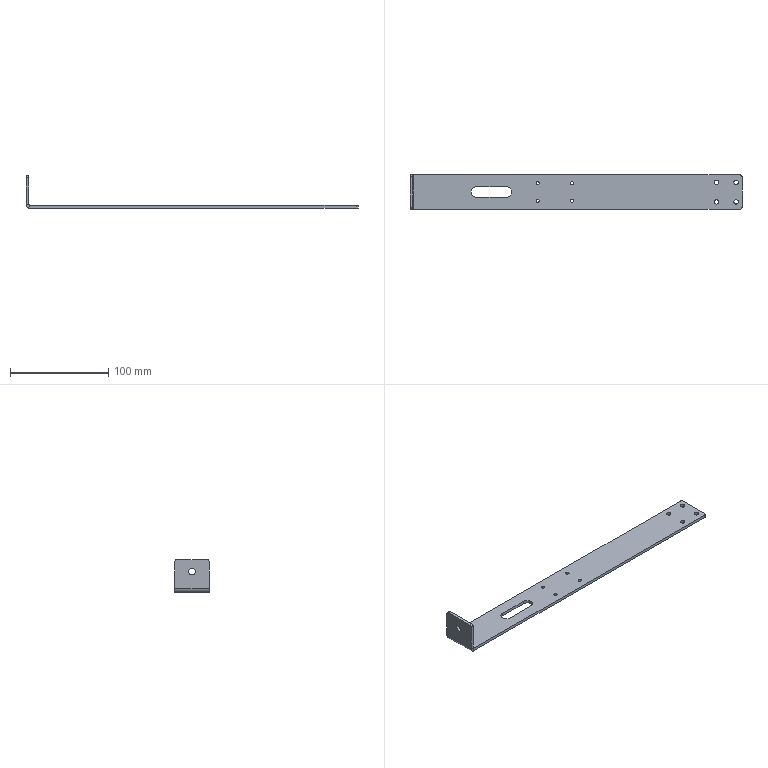Part | NX | features BREP 1 | 1 solid | 41 faces | box 338 x 35 x 33 mm | volume 36858 mm3 | cylinder 27 | plane 14 | commonest cylinder face diameters 3.3 x8 4.5 x8 4 x4 11 x3 6.6 x2 1.473 x1
STEP:
#1=CARTESIAN_POINT('',(-169.,0.,14.7));
#2=VERTEX_POINT('',#1);
#3=CARTESIAN_POINT('',(-166.,0.,14.7));
#4=VERTEX_POINT('',#3);
#5=CARTESIAN_POINT('',(-169.,0.,14.7));
#6=DIRECTION('',(-1.,0.,0.));
#7=VECTOR('',#6,1000.);
#8=LINE('',#5,#7);
#9=EDGE_CURVE('',#2,#4,#8,.F.);
#10=ORIENTED_EDGE('',*,*,#9,.T.);
#11=CARTESIAN_POINT('',(-166.,0.,21.3));
#12=VERTEX_POINT('',#11);
#13=CARTESIAN_POINT('',(-166.,0.,18.));
#14=DIRECTION('',(1.,0.,0.));
#15=DIRECTION('',(0.,0.,-1.));
#16=AXIS2_PLACEMENT_3D('',#13,#14,#15);
#17=CIRCLE('',#16,3.3);
#18=EDGE_CURVE('',#4,#12,#17,.T.);
#19=ORIENTED_EDGE('',*,*,#18,.T.);
#20=CARTESIAN_POINT('',(-169.,0.,21.3));
#21=VERTEX_POINT('',#20);
#22=CARTESIAN_POINT('',(-169.,0.,21.3));
#23=DIRECTION('',(-1.,0.,0.));
#24=VECTOR('',#23,1000.);
#25=LINE('',#22,#24);
#26=EDGE_CURVE('',#21,#12,#25,.F.);
#27=ORIENTED_EDGE('',*,*,#26,.F.);
#28=CARTESIAN_POINT('',(-169.,0.,18.));
#29=DIRECTION('',(-1.,0.,0.));
#30=DIRECTION('',(0.,0.,1.));
#31=AXIS2_PLACEMENT_3D('',#28,#29,#30);
#32=CIRCLE('',#31,3.3);
#33=EDGE_CURVE('',#21,#2,#32,.T.);
#34=ORIENTED_EDGE('',*,*,#33,.T.);
#35=EDGE_LOOP('',(#10,#19,#27,#34));
#36=FACE_BOUND('',#35,.T.);
#37=CARTESIAN_POINT('',(-169.,0.,18.));
#38=DIRECTION('',(-1.,0.,0.));
#39=DIRECTION('',(0.,0.,1.));
#40=AXIS2_PLACEMENT_3D('',#37,#38,#39);
#41=CYLINDRICAL_SURFACE('',#40,3.3);
#42=ADVANCED_FACE('',(#36),#41,.F.);
#43=CARTESIAN_POINT('',(167.,17.5,-3.));
#44=VERTEX_POINT('',#43);
#45=CARTESIAN_POINT('',(169.,15.5,-3.));
#46=VERTEX_POINT('',#45);
#47=CARTESIAN_POINT('',(167.,15.5,-3.));
#48=DIRECTION('',(0.,0.,-1.));
#49=DIRECTION('',(1.,0.,0.));
#50=AXIS2_PLACEMENT_3D('',#47,#48,#49);
#51=CIRCLE('',#50,2.);
#52=EDGE_CURVE('',#44,#46,#51,.T.);
#53=ORIENTED_EDGE('',*,*,#52,.F.);
#54=CARTESIAN_POINT('',(167.,17.5,0.));
#55=VERTEX_POINT('',#54);
#56=CARTESIAN_POINT('',(167.,17.5,-3.));
#57=DIRECTION('',(0.,0.,-1.));
#58=VECTOR('',#57,1000.);
#59=LINE('',#56,#58);
#60=EDGE_CURVE('',#55,#44,#59,.T.);
#61=ORIENTED_EDGE('',*,*,#60,.F.);
#62=CARTESIAN_POINT('',(169.,15.5,0.));
#63=VERTEX_POINT('',#62);
#64=CARTESIAN_POINT('',(167.,15.5,0.));
#65=DIRECTION('',(0.,0.,1.));
#66=DIRECTION('',(1.,0.,0.));
#67=AXIS2_PLACEMENT_3D('',#64,#65,#66);
#68=CIRCLE('',#67,2.);
#69=EDGE_CURVE('',#63,#55,#68,.T.);
#70=ORIENTED_EDGE('',*,*,#69,.F.);
#71=CARTESIAN_POINT('',(169.,15.5,-3.));
#72=DIRECTION('',(0.,0.,1.));
#73=VECTOR('',#72,1000.);
#74=LINE('',#71,#73);
#75=EDGE_CURVE('',#46,#63,#74,.T.);
#76=ORIENTED_EDGE('',*,*,#75,.F.);
#77=EDGE_LOOP('',(#53,#61,#70,#76));
#78=FACE_BOUND('',#77,.T.);
#79=CARTESIAN_POINT('',(167.,15.5,-3.));
#80=DIRECTION('',(0.,0.,1.));
#81=DIRECTION('',(1.,0.,0.));
#82=AXIS2_PLACEMENT_3D('',#79,#80,#81);
#83=CYLINDRICAL_SURFACE('',#82,2.);
#84=ADVANCED_FACE('',(#78),#83,.T.);
#85=CARTESIAN_POINT('',(169.,-15.5,-3.));
#86=VERTEX_POINT('',#85);
#87=CARTESIAN_POINT('',(167.,-17.5,-3.));
#88=VERTEX_POINT('',#87);
#89=CARTESIAN_POINT('',(167.,-15.5,-3.));
#90=DIRECTION('',(0.,0.,-1.));
#91=DIRECTION('',(1.,0.,0.));
#92=AXIS2_PLACEMENT_3D('',#89,#90,#91);
#93=CIRCLE('',#92,2.);
#94=EDGE_CURVE('',#86,#88,#93,.T.);
#95=ORIENTED_EDGE('',*,*,#94,.F.);
#96=CARTESIAN_POINT('',(169.,-15.5,0.));
#97=VERTEX_POINT('',#96);
#98=CARTESIAN_POINT('',(169.,-15.5,-3.));
#99=DIRECTION('',(0.,0.,-1.));
#100=VECTOR('',#99,1000.);
#101=LINE('',#98,#100);
#102=EDGE_CURVE('',#97,#86,#101,.T.);
#103=ORIENTED_EDGE('',*,*,#102,.F.);
#104=CARTESIAN_POINT('',(167.,-17.5,0.));
#105=VERTEX_POINT('',#104);
#106=CARTESIAN_POINT('',(167.,-15.5,0.));
#107=DIRECTION('',(0.,0.,1.));
#108=DIRECTION('',(1.,0.,0.));
#109=AXIS2_PLACEMENT_3D('',#106,#107,#108);
#110=CIRCLE('',#109,2.);
#111=EDGE_CURVE('',#105,#97,#110,.T.);
#112=ORIENTED_EDGE('',*,*,#111,.F.);
#113=CARTESIAN_POINT('',(167.,-17.5,-3.));
#114=DIRECTION('',(0.,0.,1.));
#115=VECTOR('',#114,1000.);
#116=LINE('',#113,#115);
#117=EDGE_CURVE('',#88,#105,#116,.T.);
#118=ORIENTED_EDGE('',*,*,#117,.F.);
#119=EDGE_LOOP('',(#95,#103,#112,#118));
#120=FACE_BOUND('',#119,.T.);
#121=CARTESIAN_POINT('',(167.,-15.5,-3.));
#122=DIRECTION('',(0.,0.,1.));
#123=DIRECTION('',(1.,0.,0.));
#124=AXIS2_PLACEMENT_3D('',#121,#122,#123);
#125=CYLINDRICAL_SURFACE('',#124,2.);
#126=ADVANCED_FACE('',(#120),#125,.T.);
#127=CARTESIAN_POINT('',(-169.,15.5,30.));
#128=VERTEX_POINT('',#127);
#129=CARTESIAN_POINT('',(-169.,17.5,28.));
#130=VERTEX_POINT('',#129);
#131=CARTESIAN_POINT('',(-169.,15.5,28.));
#132=DIRECTION('',(-1.,0.,0.));
#133=DIRECTION('',(0.,0.,-1.));
#134=AXIS2_PLACEMENT_3D('',#131,#132,#133);
#135=CIRCLE('',#134,2.);
#136=EDGE_CURVE('',#128,#130,#135,.T.);
#137=ORIENTED_EDGE('',*,*,#136,.F.);
#138=CARTESIAN_POINT('',(-166.,15.5,30.));
#139=VERTEX_POINT('',#138);
#140=CARTESIAN_POINT('',(-169.,15.5,30.));
#141=DIRECTION('',(-1.,0.,0.));
#142=VECTOR('',#141,1000.);
#143=LINE('',#140,#142);
#144=EDGE_CURVE('',#139,#128,#143,.T.);
#145=ORIENTED_EDGE('',*,*,#144,.F.);
#146=CARTESIAN_POINT('',(-166.,17.5,28.));
#147=VERTEX_POINT('',#146);
#148=CARTESIAN_POINT('',(-166.,15.5,28.));
#149=DIRECTION('',(1.,0.,0.));
#150=DIRECTION('',(0.,0.,-1.));
#151=AXIS2_PLACEMENT_3D('',#148,#149,#150);
#152=CIRCLE('',#151,2.);
#153=EDGE_CURVE('',#147,#139,#152,.T.);
#154=ORIENTED_EDGE('',*,*,#153,.F.);
#155=CARTESIAN_POINT('',(-169.,17.5,28.));
#156=DIRECTION('',(1.,0.,0.));
#157=VECTOR('',#156,1000.);
#158=LINE('',#155,#157);
#159=EDGE_CURVE('',#130,#147,#158,.T.);
#160=ORIENTED_EDGE('',*,*,#159,.F.);
#161=EDGE_LOOP('',(#137,#145,#154,#160));
#162=FACE_BOUND('',#161,.T.);
#163=CARTESIAN_POINT('',(-169.,15.5,28.));
#164=DIRECTION('',(1.,0.,0.));
#165=DIRECTION('',(0.,0.,-1.));
#166=AXIS2_PLACEMENT_3D('',#163,#164,#165);
#167=CYLINDRICAL_SURFACE('',#166,2.);
#168=ADVANCED_FACE('',(#162),#167,.T.);
#169=CARTESIAN_POINT('',(-169.,-17.5,28.));
#170=VERTEX_POINT('',#169);
#171=CARTESIAN_POINT('',(-169.,-15.5,30.));
#172=VERTEX_POINT('',#171);
#173=CARTESIAN_POINT('',(-169.,-15.5,28.));
#174=DIRECTION('',(-1.,0.,0.));
#175=DIRECTION('',(0.,0.,-1.));
#176=AXIS2_PLACEMENT_3D('',#173,#174,#175);
#177=CIRCLE('',#176,2.);
#178=EDGE_CURVE('',#170,#172,#177,.T.);
#179=ORIENTED_EDGE('',*,*,#178,.F.);
#180=CARTESIAN_POINT('',(-166.,-17.5,28.));
#181=VERTEX_POINT('',#180);
#182=CARTESIAN_POINT('',(-169.,-17.5,28.));
#183=DIRECTION('',(-1.,0.,0.));
#184=VECTOR('',#183,1000.);
#185=LINE('',#182,#184);
#186=EDGE_CURVE('',#181,#170,#185,.T.);
#187=ORIENTED_EDGE('',*,*,#186,.F.);
#188=CARTESIAN_POINT('',(-166.,-15.5,30.));
#189=VERTEX_POINT('',#188);
#190=CARTESIAN_POINT('',(-166.,-15.5,28.));
#191=DIRECTION('',(1.,0.,0.));
#192=DIRECTION('',(0.,0.,-1.));
#193=AXIS2_PLACEMENT_3D('',#190,#191,#192);
#194=CIRCLE('',#193,2.);
#195=EDGE_CURVE('',#189,#181,#194,.T.);
#196=ORIENTED_EDGE('',*,*,#195,.F.);
#197=CARTESIAN_POINT('',(-169.,-15.5,30.));
#198=DIRECTION('',(1.,0.,0.));
#199=VECTOR('',#198,1000.);
#200=LINE('',#197,#199);
#201=EDGE_CURVE('',#172,#189,#200,.T.);
#202=ORIENTED_EDGE('',*,*,#201,.F.);
#203=EDGE_LOOP('',(#179,#187,#196,#202));
#204=FACE_BOUND('',#203,.T.);
#205=CARTESIAN_POINT('',(-169.,-15.5,28.));
#206=DIRECTION('',(1.,0.,0.));
#207=DIRECTION('',(0.,0.,-1.));
#208=AXIS2_PLACEMENT_3D('',#205,#206,#207);
#209=CYLINDRICAL_SURFACE('',#208,2.);
#210=ADVANCED_FACE('',(#204),#209,.T.);
#211=CARTESIAN_POINT('',(-71.,5.5,0.));
#212=VERTEX_POINT('',#211);
#213=CARTESIAN_POINT('',(-101.,5.5,0.));
#214=VERTEX_POINT('',#213);
#215=CARTESIAN_POINT('',(0.,5.5,0.));
#216=DIRECTION('',(-1.,0.,0.));
#217=VECTOR('',#216,1000.);
#218=LINE('',#215,#217);
#219=EDGE_CURVE('',#212,#214,#218,.T.);
#220=ORIENTED_EDGE('',*,*,#219,.T.);
#221=CARTESIAN_POINT('',(-101.,5.5,-3.));
#222=VERTEX_POINT('',#221);
#223=CARTESIAN_POINT('',(-101.,5.5,-3.));
#224=DIRECTION('',(0.,0.,-1.));
#225=VECTOR('',#224,1000.);
#226=LINE('',#223,#225);
#227=EDGE_CURVE('',#214,#222,#226,.T.);
#228=ORIENTED_EDGE('',*,*,#227,.T.);
#229=CARTESIAN_POINT('',(-71.,5.5,-3.));
#230=VERTEX_POINT('',#229);
#231=CARTESIAN_POINT('',(-101.,5.5,-3.));
#232=DIRECTION('',(1.,0.,0.));
#233=VECTOR('',#232,1000.);
#234=LINE('',#231,#233);
#235=EDGE_CURVE('',#222,#230,#234,.T.);
#236=ORIENTED_EDGE('',*,*,#235,.T.);
#237=CARTESIAN_POINT('',(-71.,5.5,-3.));
#238=DIRECTION('',(0.,0.,1.));
#239=VECTOR('',#238,1000.);
#240=LINE('',#237,#239);
#241=EDGE_CURVE('',#230,#212,#240,.T.);
#242=ORIENTED_EDGE('',*,*,#241,.T.);
#243=EDGE_LOOP('',(#220,#228,#236,#242));
#244=FACE_BOUND('',#243,.T.);
#245=CARTESIAN_POINT('',(-101.,5.5,-3.));
#246=DIRECTION('',(0.,1.,0.));
#247=DIRECTION('',(0.,0.,1.));
#248=AXIS2_PLACEMENT_3D('',#245,#246,#247);
#249=PLANE('',#248);
#250=ADVANCED_FACE('',(#244),#249,.F.);
#251=CARTESIAN_POINT('',(-101.,-5.5,0.));
#252=VERTEX_POINT('',#251);
#253=CARTESIAN_POINT('',(-71.,-5.5,0.));
#254=VERTEX_POINT('',#253);
#255=CARTESIAN_POINT('',(0.,-5.5,0.));
#256=DIRECTION('',(1.,0.,0.));
#257=VECTOR('',#256,1000.);
#258=LINE('',#255,#257);
#259=EDGE_CURVE('',#252,#254,#258,.T.);
#260=ORIENTED_EDGE('',*,*,#259,.T.);
#261=CARTESIAN_POINT('',(-71.,-5.5,-3.));
#262=VERTEX_POINT('',#261);
#263=CARTESIAN_POINT('',(-71.,-5.5,-3.));
#264=DIRECTION('',(0.,0.,-1.));
#265=VECTOR('',#264,1000.);
#266=LINE('',#263,#265);
#267=EDGE_CURVE('',#254,#262,#266,.T.);
#268=ORIENTED_EDGE('',*,*,#267,.T.);
#269=CARTESIAN_POINT('',(-101.,-5.5,-3.));
#270=VERTEX_POINT('',#269);
#271=CARTESIAN_POINT('',(-101.,-5.5,-3.));
#272=DIRECTION('',(1.,0.,0.));
#273=VECTOR('',#272,1000.);
#274=LINE('',#271,#273);
#275=EDGE_CURVE('',#270,#262,#274,.T.);
#276=ORIENTED_EDGE('',*,*,#275,.F.);
#277=CARTESIAN_POINT('',(-101.,-5.5,-3.));
#278=DIRECTION('',(0.,0.,1.));
#279=VECTOR('',#278,1000.);
#280=LINE('',#277,#279);
#281=EDGE_CURVE('',#270,#252,#280,.T.);
#282=ORIENTED_EDGE('',*,*,#281,.T.);
#283=EDGE_LOOP('',(#260,#268,#276,#282));
#284=FACE_BOUND('',#283,.T.);
#285=CARTESIAN_POINT('',(-101.,-5.5,-3.));
#286=DIRECTION('',(0.,-1.,0.));
#287=DIRECTION('',(0.,0.,-1.));
#288=AXIS2_PLACEMENT_3D('',#285,#286,#287);
#289=PLANE('',#288);
#290=ADVANCED_FACE('',(#284),#289,.F.);
#291=CARTESIAN_POINT('',(-106.5,0.,0.));
#292=VERTEX_POINT('',#291);
#293=CARTESIAN_POINT('',(-106.5,0.,-3.));
#294=VERTEX_POINT('',#293);
#295=CARTESIAN_POINT('',(-106.5,0.,-3.));
#296=DIRECTION('',(0.,0.,-1.));
#297=VECTOR('',#296,1000.);
#298=LINE('',#295,#297);
#299=EDGE_CURVE('',#292,#294,#298,.T.);
#300=ORIENTED_EDGE('',*,*,#299,.F.);
#301=CARTESIAN_POINT('',(-101.,0.,0.));
#302=DIRECTION('',(0.,0.,1.));
#303=DIRECTION('',(1.,0.,0.));
#304=AXIS2_PLACEMENT_3D('',#301,#302,#303);
#305=CIRCLE('',#304,5.5);
#306=EDGE_CURVE('',#292,#252,#305,.T.);
#307=ORIENTED_EDGE('',*,*,#306,.T.);
#308=ORIENTED_EDGE('',*,*,#281,.F.);
#309=CARTESIAN_POINT('',(-101.,0.,-3.));
#310=DIRECTION('',(0.,0.,-1.));
#311=DIRECTION('',(-1.,0.,0.));
#312=AXIS2_PLACEMENT_3D('',#309,#310,#311);
#313=CIRCLE('',#312,5.5);
#314=EDGE_CURVE('',#270,#294,#313,.T.);
#315=ORIENTED_EDGE('',*,*,#314,.T.);
#316=EDGE_LOOP('',(#300,#307,#308,#315));
#317=FACE_BOUND('',#316,.T.);
#318=CARTESIAN_POINT('',(-101.,0.,-3.));
#319=DIRECTION('',(0.,0.,-1.));
#320=DIRECTION('',(-1.,0.,0.));
#321=AXIS2_PLACEMENT_3D('',#318,#319,#320);
#322=CYLINDRICAL_SURFACE('',#321,5.5);
#323=ADVANCED_FACE('',(#317),#322,.F.);
#324=CARTESIAN_POINT('',(-71.,0.,0.));
#325=DIRECTION('',(0.,0.,1.));
#326=DIRECTION('',(1.,0.,0.));
#327=AXIS2_PLACEMENT_3D('',#324,#325,#326);
#328=CIRCLE('',#327,5.5);
#329=EDGE_CURVE('',#254,#212,#328,.T.);
#330=ORIENTED_EDGE('',*,*,#329,.T.);
#331=ORIENTED_EDGE('',*,*,#241,.F.);
#332=CARTESIAN_POINT('',(-71.,0.,-3.));
#333=DIRECTION('',(0.,0.,-1.));
#334=DIRECTION('',(-1.,0.,0.));
#335=AXIS2_PLACEMENT_3D('',#332,#333,#334);
#336=CIRCLE('',#335,5.5);
#337=EDGE_CURVE('',#230,#262,#336,.T.);
#338=ORIENTED_EDGE('',*,*,#337,.T.);
#339=ORIENTED_EDGE('',*,*,#267,.F.);
#340=EDGE_LOOP('',(#330,#331,#338,#339));
#341=FACE_BOUND('',#340,.T.);
#342=CARTESIAN_POINT('',(-71.,0.,-3.));
#343=DIRECTION('',(0.,0.,-1.));
#344=DIRECTION('',(-1.,0.,0.));
#345=AXIS2_PLACEMENT_3D('',#342,#343,#344);
#346=CYLINDRICAL_SURFACE('',#345,5.5);
#347=ADVANCED_FACE('',(#341),#346,.F.);
#348=CARTESIAN_POINT('',(-40.65,9.,0.));
#349=VERTEX_POINT('',#348);
#350=CARTESIAN_POINT('',(-40.65,9.,-3.));
#351=VERTEX_POINT('',#350);
#352=CARTESIAN_POINT('',(-40.65,9.,0.));
#353=DIRECTION('',(0.,0.,1.));
#354=VECTOR('',#353,1000.);
#355=LINE('',#352,#354);
#356=EDGE_CURVE('',#349,#351,#355,.F.);
#357=ORIENTED_EDGE('',*,*,#356,.T.);
#358=CARTESIAN_POINT('',(-37.35,9.,-3.));
#359=VERTEX_POINT('',#358);
#360=CARTESIAN_POINT('',(-39.,9.,-3.));
#361=DIRECTION('',(0.,0.,1.));
#362=DIRECTION('',(1.,0.,0.));
#363=AXIS2_PLACEMENT_3D('',#360,#361,#362);
#364=CIRCLE('',#363,1.65);
#365=EDGE_CURVE('',#359,#351,#364,.T.);
#366=ORIENTED_EDGE('',*,*,#365,.F.);
#367=CARTESIAN_POINT('',(-37.35,9.,0.));
#368=VERTEX_POINT('',#367);
#369=CARTESIAN_POINT('',(-37.35,9.,0.));
#370=DIRECTION('',(0.,0.,1.));
#371=VECTOR('',#370,1000.);
#372=LINE('',#369,#371);
#373=EDGE_CURVE('',#368,#359,#372,.F.);
#374=ORIENTED_EDGE('',*,*,#373,.F.);
#375=CARTESIAN_POINT('',(-39.,9.,0.));
#376=DIRECTION('',(0.,0.,1.));
#377=DIRECTION('',(1.,0.,0.));
#378=AXIS2_PLACEMENT_3D('',#375,#376,#377);
#379=CIRCLE('',#378,1.65);
#380=EDGE_CURVE('',#368,#349,#379,.T.);
#381=ORIENTED_EDGE('',*,*,#380,.T.);
#382=EDGE_LOOP('',(#357,#366,#374,#381));
#383=FACE_BOUND('',#382,.T.);
#384=CARTESIAN_POINT('',(-39.,9.,0.));
#385=DIRECTION('',(0.,0.,1.));
#386=DIRECTION('',(1.,0.,0.));
#387=AXIS2_PLACEMENT_3D('',#384,#385,#386);
#388=CYLINDRICAL_SURFACE('',#387,1.65);
#389=ADVANCED_FACE('',(#383),#388,.F.);
#390=CARTESIAN_POINT('',(-40.65,-9.,0.));
#391=VERTEX_POINT('',#390);
#392=CARTESIAN_POINT('',(-40.65,-9.,-3.));
#393=VERTEX_POINT('',#392);
#394=CARTESIAN_POINT('',(-40.65,-9.,0.));
#395=DIRECTION('',(0.,0.,1.));
#396=VECTOR('',#395,1000.);
#397=LINE('',#394,#396);
#398=EDGE_CURVE('',#391,#393,#397,.F.);
#399=ORIENTED_EDGE('',*,*,#398,.T.);
#400=CARTESIAN_POINT('',(-37.35,-9.,-3.));
#401=VERTEX_POINT('',#400);
#402=CARTESIAN_POINT('',(-39.,-9.,-3.));
#403=DIRECTION('',(0.,0.,1.));
#404=DIRECTION('',(1.,0.,0.));
#405=AXIS2_PLACEMENT_3D('',#402,#403,#404);
#406=CIRCLE('',#405,1.65);
#407=EDGE_CURVE('',#401,#393,#406,.T.);
#408=ORIENTED_EDGE('',*,*,#407,.F.);
#409=CARTESIAN_POINT('',(-37.35,-9.,0.));
#410=VERTEX_POINT('',#409);
#411=CARTESIAN_POINT('',(-37.35,-9.,0.));
#412=DIRECTION('',(0.,0.,1.));
#413=VECTOR('',#412,1000.);
#414=LINE('',#411,#413);
#415=EDGE_CURVE('',#410,#401,#414,.F.);
#416=ORIENTED_EDGE('',*,*,#415,.F.);
#417=CARTESIAN_POINT('',(-39.,-9.,0.));
#418=DIRECTION('',(0.,0.,1.));
#419=DIRECTION('',(1.,0.,0.));
#420=AXIS2_PLACEMENT_3D('',#417,#418,#419);
#421=CIRCLE('',#420,1.65);
#422=EDGE_CURVE('',#410,#391,#421,.T.);
#423=ORIENTED_EDGE('',*,*,#422,.T.);
#424=EDGE_LOOP('',(#399,#408,#416,#423));
#425=FACE_BOUND('',#424,.T.);
#426=CARTESIAN_POINT('',(-39.,-9.,0.));
#427=DIRECTION('',(0.,0.,1.));
#428=DIRECTION('',(1.,0.,0.));
#429=AXIS2_PLACEMENT_3D('',#426,#427,#428);
#430=CYLINDRICAL_SURFACE('',#429,1.65);
#431=ADVANCED_FACE('',(#425),#430,.F.);
#432=CARTESIAN_POINT('',(-5.65,-9.,0.));
#433=VERTEX_POINT('',#432);
#434=CARTESIAN_POINT('',(-5.65,-9.,-3.));
#435=VERTEX_POINT('',#434);
#436=CARTESIAN_POINT('',(-5.65,-9.,0.));
#437=DIRECTION('',(0.,0.,1.));
#438=VECTOR('',#437,1000.);
#439=LINE('',#436,#438);
#440=EDGE_CURVE('',#433,#435,#439,.F.);
#441=ORIENTED_EDGE('',*,*,#440,.T.);
#442=CARTESIAN_POINT('',(-2.35,-9.,-3.));
#443=VERTEX_POINT('',#442);
#444=CARTESIAN_POINT('',(-4.,-9.,-3.));
#445=DIRECTION('',(0.,0.,1.));
#446=DIRECTION('',(1.,0.,0.));
#447=AXIS2_PLACEMENT_3D('',#444,#445,#446);
#448=CIRCLE('',#447,1.65);
#449=EDGE_CURVE('',#443,#435,#448,.T.);
#450=ORIENTED_EDGE('',*,*,#449,.F.);
#451=CARTESIAN_POINT('',(-2.35,-9.,0.));
#452=VERTEX_POINT('',#451);
#453=CARTESIAN_POINT('',(-2.35,-9.,0.));
#454=DIRECTION('',(0.,0.,1.));
#455=VECTOR('',#454,1000.);
#456=LINE('',#453,#455);
#457=EDGE_CURVE('',#452,#443,#456,.F.);
#458=ORIENTED_EDGE('',*,*,#457,.F.);
#459=CARTESIAN_POINT('',(-4.,-9.,0.));
#460=DIRECTION('',(0.,0.,1.));
#461=DIRECTION('',(1.,0.,0.));
#462=AXIS2_PLACEMENT_3D('',#459,#460,#461);
#463=CIRCLE('',#462,1.65);
#464=EDGE_CURVE('',#452,#433,#463,.T.);
#465=ORIENTED_EDGE('',*,*,#464,.T.);
#466=EDGE_LOOP('',(#441,#450,#458,#465));
#467=FACE_BOUND('',#466,.T.);
#468=CARTESIAN_POINT('',(-4.,-9.,0.));
#469=DIRECTION('',(0.,0.,1.));
#470=DIRECTION('',(1.,0.,0.));
#471=AXIS2_PLACEMENT_3D('',#468,#469,#470);
#472=CYLINDRICAL_SURFACE('',#471,1.65);
#473=ADVANCED_FACE('',(#467),#472,.F.);
#474=CARTESIAN_POINT('',(-5.65,9.,0.));
#475=VERTEX_POINT('',#474);
#476=CARTESIAN_POINT('',(-5.65,9.,-3.));
#477=VERTEX_POINT('',#476);
#478=CARTESIAN_POINT('',(-5.65,9.,0.));
#479=DIRECTION('',(0.,0.,1.));
#480=VECTOR('',#479,1000.);
#481=LINE('',#478,#480);
#482=EDGE_CURVE('',#475,#477,#481,.F.);
#483=ORIENTED_EDGE('',*,*,#482,.T.);
#484=CARTESIAN_POINT('',(-2.35,9.,-3.));
#485=VERTEX_POINT('',#484);
#486=CARTESIAN_POINT('',(-4.,9.,-3.));
#487=DIRECTION('',(0.,0.,1.));
#488=DIRECTION('',(1.,0.,0.));
#489=AXIS2_PLACEMENT_3D('',#486,#487,#488);
#490=CIRCLE('',#489,1.65);
#491=EDGE_CURVE('',#485,#477,#490,.T.);
#492=ORIENTED_EDGE('',*,*,#491,.F.);
#493=CARTESIAN_POINT('',(-2.35,9.,0.));
#494=VERTEX_POINT('',#493);
#495=CARTESIAN_POINT('',(-2.35,9.,0.));
#496=DIRECTION('',(0.,0.,1.));
#497=VECTOR('',#496,1000.);
#498=LINE('',#495,#497);
#499=EDGE_CURVE('',#494,#485,#498,.F.);
#500=ORIENTED_EDGE('',*,*,#499,.F.);
#501=CARTESIAN_POINT('',(-4.,9.,0.));
#502=DIRECTION('',(0.,0.,1.));
#503=DIRECTION('',(1.,0.,0.));
#504=AXIS2_PLACEMENT_3D('',#501,#502,#503);
#505=CIRCLE('',#504,1.65);
#506=EDGE_CURVE('',#494,#475,#505,.T.);
#507=ORIENTED_EDGE('',*,*,#506,.T.);
#508=EDGE_LOOP('',(#483,#492,#500,#507));
#509=FACE_BOUND('',#508,.T.);
#510=CARTESIAN_POINT('',(-4.,9.,0.));
#511=DIRECTION('',(0.,0.,1.));
#512=DIRECTION('',(1.,0.,0.));
#513=AXIS2_PLACEMENT_3D('',#510,#511,#512);
#514=CYLINDRICAL_SURFACE('',#513,1.65);
#515=ADVANCED_FACE('',(#509),#514,.F.);
#516=CARTESIAN_POINT('',(140.75,10.,0.));
#517=VERTEX_POINT('',#516);
#518=CARTESIAN_POINT('',(140.75,10.,-3.));
#519=VERTEX_POINT('',#518);
#520=CARTESIAN_POINT('',(140.75,10.,0.));
#521=DIRECTION('',(0.,0.,1.));
#522=VECTOR('',#521,1000.);
#523=LINE('',#520,#522);
#524=EDGE_CURVE('',#517,#519,#523,.F.);
#525=ORIENTED_EDGE('',*,*,#524,.T.);
#526=CARTESIAN_POINT('',(145.25,10.,-3.));
#527=VERTEX_POINT('',#526);
#528=CARTESIAN_POINT('',(143.,10.,-3.));
#529=DIRECTION('',(0.,0.,1.));
#530=DIRECTION('',(1.,0.,0.));
#531=AXIS2_PLACEMENT_3D('',#528,#529,#530);
#532=CIRCLE('',#531,2.25);
#533=EDGE_CURVE('',#527,#519,#532,.T.);
#534=ORIENTED_EDGE('',*,*,#533,.F.);
#535=CARTESIAN_POINT('',(145.25,10.,0.));
#536=VERTEX_POINT('',#535);
#537=CARTESIAN_POINT('',(145.25,10.,0.));
#538=DIRECTION('',(0.,0.,1.));
#539=VECTOR('',#538,1000.);
#540=LINE('',#537,#539);
#541=EDGE_CURVE('',#536,#527,#540,.F.);
#542=ORIENTED_EDGE('',*,*,#541,.F.);
#543=CARTESIAN_POINT('',(143.,10.,0.));
#544=DIRECTION('',(0.,0.,1.));
#545=DIRECTION('',(1.,0.,0.));
#546=AXIS2_PLACEMENT_3D('',#543,#544,#545);
#547=CIRCLE('',#546,2.25);
#548=EDGE_CURVE('',#536,#517,#547,.T.);
#549=ORIENTED_EDGE('',*,*,#548,.T.);
#550=EDGE_LOOP('',(#525,#534,#542,#549));
#551=FACE_BOUND('',#550,.T.);
#552=CARTESIAN_POINT('',(143.,10.,0.));
#553=DIRECTION('',(0.,0.,1.));
#554=DIRECTION('',(1.,0.,0.));
#555=AXIS2_PLACEMENT_3D('',#552,#553,#554);
#556=CYLINDRICAL_SURFACE('',#555,2.25);
#557=ADVANCED_FACE('',(#551),#556,.F.);
#558=CARTESIAN_POINT('',(160.75,-10.,0.));
#559=VERTEX_POINT('',#558);
#560=CARTESIAN_POINT('',(160.75,-10.,-3.));
#561=VERTEX_POINT('',#560);
#562=CARTESIAN_POINT('',(160.75,-10.,0.));
#563=DIRECTION('',(0.,0.,1.));
#564=VECTOR('',#563,1000.);
#565=LINE('',#562,#564);
#566=EDGE_CURVE('',#559,#561,#565,.F.);
#567=ORIENTED_EDGE('',*,*,#566,.T.);
#568=CARTESIAN_POINT('',(165.25,-10.,-3.));
#569=VERTEX_POINT('',#568);
#570=CARTESIAN_POINT('',(163.,-10.,-3.));
#571=DIRECTION('',(0.,0.,1.));
#572=DIRECTION('',(1.,0.,0.));
#573=AXIS2_PLACEMENT_3D('',#570,#571,#572);
#574=CIRCLE('',#573,2.25);
#575=EDGE_CURVE('',#569,#561,#574,.T.);
#576=ORIENTED_EDGE('',*,*,#575,.F.);
#577=CARTESIAN_POINT('',(165.25,-10.,0.));
#578=VERTEX_POINT('',#577);
#579=CARTESIAN_POINT('',(165.25,-10.,0.));
#580=DIRECTION('',(0.,0.,1.));
#581=VECTOR('',#580,1000.);
#582=LINE('',#579,#581);
#583=EDGE_CURVE('',#578,#569,#582,.F.);
#584=ORIENTED_EDGE('',*,*,#583,.F.);
#585=CARTESIAN_POINT('',(163.,-10.,0.));
#586=DIRECTION('',(0.,0.,1.));
#587=DIRECTION('',(1.,0.,0.));
#588=AXIS2_PLACEMENT_3D('',#585,#586,#587);
#589=CIRCLE('',#588,2.25);
#590=EDGE_CURVE('',#578,#559,#589,.T.);
#591=ORIENTED_EDGE('',*,*,#590,.T.);
#592=EDGE_LOOP('',(#567,#576,#584,#591));
#593=FACE_BOUND('',#592,.T.);
#594=CARTESIAN_POINT('',(163.,-10.,0.));
#595=DIRECTION('',(0.,0.,1.));
#596=DIRECTION('',(1.,0.,0.));
#597=AXIS2_PLACEMENT_3D('',#594,#595,#596);
#598=CYLINDRICAL_SURFACE('',#597,2.25);
#599=ADVANCED_FACE('',(#593),#598,.F.);
#600=CARTESIAN_POINT('',(140.75,-10.,0.));
#601=VERTEX_POINT('',#600);
#602=CARTESIAN_POINT('',(140.75,-10.,-3.));
#603=VERTEX_POINT('',#602);
#604=CARTESIAN_POINT('',(140.75,-10.,0.));
#605=DIRECTION('',(0.,0.,1.));
#606=VECTOR('',#605,1000.);
#607=LINE('',#604,#606);
#608=EDGE_CURVE('',#601,#603,#607,.F.);
#609=ORIENTED_EDGE('',*,*,#608,.T.);
#610=CARTESIAN_POINT('',(145.25,-10.,-3.));
#611=VERTEX_POINT('',#610);
#612=CARTESIAN_POINT('',(143.,-10.,-3.));
#613=DIRECTION('',(0.,0.,1.));
#614=DIRECTION('',(1.,0.,0.));
#615=AXIS2_PLACEMENT_3D('',#612,#613,#614);
#616=CIRCLE('',#615,2.25);
#617=EDGE_CURVE('',#611,#603,#616,.T.);
#618=ORIENTED_EDGE('',*,*,#617,.F.);
#619=CARTESIAN_POINT('',(145.25,-10.,0.));
#620=VERTEX_POINT('',#619);
#621=CARTESIAN_POINT('',(145.25,-10.,0.));
#622=DIRECTION('',(0.,0.,1.));
#623=VECTOR('',#622,1000.);
#624=LINE('',#621,#623);
#625=EDGE_CURVE('',#620,#611,#624,.F.);
#626=ORIENTED_EDGE('',*,*,#625,.F.);
#627=CARTESIAN_POINT('',(143.,-10.,0.));
#628=DIRECTION('',(0.,0.,1.));
#629=DIRECTION('',(1.,0.,0.));
#630=AXIS2_PLACEMENT_3D('',#627,#628,#629);
#631=CIRCLE('',#630,2.25);
#632=EDGE_CURVE('',#620,#601,#631,.T.);
#633=ORIENTED_EDGE('',*,*,#632,.T.);
#634=EDGE_LOOP('',(#609,#618,#626,#633));
#635=FACE_BOUND('',#634,.T.);
#636=CARTESIAN_POINT('',(143.,-10.,0.));
#637=DIRECTION('',(0.,0.,1.));
#638=DIRECTION('',(1.,0.,0.));
#639=AXIS2_PLACEMENT_3D('',#636,#637,#638);
#640=CYLINDRICAL_SURFACE('',#639,2.25);
#641=ADVANCED_FACE('',(#635),#640,.F.);
#642=CARTESIAN_POINT('',(160.75,10.,0.));
#643=VERTEX_POINT('',#642);
#644=CARTESIAN_POINT('',(160.75,10.,-3.));
#645=VERTEX_POINT('',#644);
#646=CARTESIAN_POINT('',(160.75,10.,0.));
#647=DIRECTION('',(0.,0.,1.));
#648=VECTOR('',#647,1000.);
#649=LINE('',#646,#648);
#650=EDGE_CURVE('',#643,#645,#649,.F.);
#651=ORIENTED_EDGE('',*,*,#650,.T.);
#652=CARTESIAN_POINT('',(165.25,10.,-3.));
#653=VERTEX_POINT('',#652);
#654=CARTESIAN_POINT('',(163.,10.,-3.));
#655=DIRECTION('',(0.,0.,1.));
#656=DIRECTION('',(1.,0.,0.));
#657=AXIS2_PLACEMENT_3D('',#654,#655,#656);
#658=CIRCLE('',#657,2.25);
#659=EDGE_CURVE('',#653,#645,#658,.T.);
#660=ORIENTED_EDGE('',*,*,#659,.F.);
#661=CARTESIAN_POINT('',(165.25,10.,0.));
#662=VERTEX_POINT('',#661);
#663=CARTESIAN_POINT('',(165.25,10.,0.));
#664=DIRECTION('',(0.,0.,1.));
#665=VECTOR('',#664,1000.);
#666=LINE('',#663,#665);
#667=EDGE_CURVE('',#662,#653,#666,.F.);
#668=ORIENTED_EDGE('',*,*,#667,.F.);
#669=CARTESIAN_POINT('',(163.,10.,0.));
#670=DIRECTION('',(0.,0.,1.));
#671=DIRECTION('',(1.,0.,0.));
#672=AXIS2_PLACEMENT_3D('',#669,#670,#671);
#673=CIRCLE('',#672,2.25);
#674=EDGE_CURVE('',#662,#643,#673,.T.);
#675=ORIENTED_EDGE('',*,*,#674,.T.);
#676=EDGE_LOOP('',(#651,#660,#668,#675));
#677=FACE_BOUND('',#676,.T.);
#678=CARTESIAN_POINT('',(163.,10.,0.));
#679=DIRECTION('',(0.,0.,1.));
#680=DIRECTION('',(1.,0.,0.));
#681=AXIS2_PLACEMENT_3D('',#678,#679,#680);
#682=CYLINDRICAL_SURFACE('',#681,2.25);
#683=ADVANCED_FACE('',(#677),#682,.F.);
#684=CARTESIAN_POINT('',(-169.,0.,30.));
#685=DIRECTION('',(0.,1.,0.));
#686=VECTOR('',#685,1000.);
#687=LINE('',#684,#686);
#688=EDGE_CURVE('',#172,#128,#687,.T.);
#689=ORIENTED_EDGE('',*,*,#688,.F.);
#690=ORIENTED_EDGE('',*,*,#201,.T.);
#691=CARTESIAN_POINT('',(-166.,17.5,30.));
#692=DIRECTION('',(0.,1.,0.));
#693=VECTOR('',#692,1000.);
#694=LINE('',#691,#693);
#695=EDGE_CURVE('',#189,#139,#694,.T.);
#696=ORIENTED_EDGE('',*,*,#695,.T.);
#697=ORIENTED_EDGE('',*,*,#144,.T.);
#698=EDGE_LOOP('',(#689,#690,#696,#697));
#699=FACE_BOUND('',#698,.T.);
#700=CARTESIAN_POINT('',(-169.,17.5,30.));
#701=DIRECTION('',(0.,0.,-1.));
#702=DIRECTION('',(-1.,0.,0.));
#703=AXIS2_PLACEMENT_3D('',#700,#701,#702);
#704=PLANE('',#703);
#705=ADVANCED_FACE('',(#699),#704,.F.);
#706=ORIENTED_EDGE('',*,*,#695,.F.);
#707=ORIENTED_EDGE('',*,*,#195,.T.);
#708=CARTESIAN_POINT('',(-166.,-17.5,0.7366));
#709=VERTEX_POINT('',#708);
#710=CARTESIAN_POINT('',(-166.,-17.5,30.));
#711=DIRECTION('',(0.,0.,1.));
#712=VECTOR('',#711,1000.);
#713=LINE('',#710,#712);
#714=EDGE_CURVE('',#709,#181,#713,.T.);
#715=ORIENTED_EDGE('',*,*,#714,.F.);
#716=CARTESIAN_POINT('',(-166.,17.5,0.7366));
#717=VERTEX_POINT('',#716);
#718=CARTESIAN_POINT('',(-166.,17.5,0.7366));
#719=DIRECTION('',(0.,-1.,0.));
#720=VECTOR('',#719,1000.);
#721=LINE('',#718,#720);
#722=EDGE_CURVE('',#717,#709,#721,.T.);
#723=ORIENTED_EDGE('',*,*,#722,.F.);
#724=CARTESIAN_POINT('',(-166.,17.5,0.));
#725=DIRECTION('',(0.,0.,-1.));
#726=VECTOR('',#725,1000.);
#727=LINE('',#724,#726);
#728=EDGE_CURVE('',#147,#717,#727,.T.);
#729=ORIENTED_EDGE('',*,*,#728,.F.);
#730=ORIENTED_EDGE('',*,*,#153,.T.);
#731=EDGE_LOOP('',(#706,#707,#715,#723,#729,#730));
#732=FACE_BOUND('',#731,.T.);
#733=CARTESIAN_POINT('',(-166.,0.,18.));
#734=DIRECTION('',(1.,0.,0.));
#735=DIRECTION('',(0.,0.,-1.));
#736=AXIS2_PLACEMENT_3D('',#733,#734,#735);
#737=CIRCLE('',#736,3.3);
#738=EDGE_CURVE('',#12,#4,#737,.T.);
#739=ORIENTED_EDGE('',*,*,#738,.F.);
#740=ORIENTED_EDGE('',*,*,#18,.F.);
#741=EDGE_LOOP('',(#739,#740));
#742=FACE_BOUND('',#741,.T.);
#743=CARTESIAN_POINT('',(-166.,0.,0.));
#744=DIRECTION('',(1.,0.,0.));
#745=DIRECTION('',(0.,0.,-1.));
#746=AXIS2_PLACEMENT_3D('',#743,#744,#745);
#747=PLANE('',#746);
#748=ADVANCED_FACE('',(#732,#742),#747,.T.);
#749=CARTESIAN_POINT('',(-169.,17.5,0.7366));
#750=VERTEX_POINT('',#749);
#751=CARTESIAN_POINT('',(-169.,17.5,0.));
#752=DIRECTION('',(0.,0.,-1.));
#753=VECTOR('',#752,1000.);
#754=LINE('',#751,#753);
#755=EDGE_CURVE('',#130,#750,#754,.T.);
#756=ORIENTED_EDGE('',*,*,#755,.F.);
#757=ORIENTED_EDGE('',*,*,#159,.T.);
#758=ORIENTED_EDGE('',*,*,#728,.T.);
#759=CARTESIAN_POINT('',(-169.,17.5,0.7366));
#760=DIRECTION('',(-1.,0.,0.));
#761=VECTOR('',#760,1000.);
#762=LINE('',#759,#761);
#763=EDGE_CURVE('',#717,#750,#762,.T.);
#764=ORIENTED_EDGE('',*,*,#763,.T.);
#765=EDGE_LOOP('',(#756,#757,#758,#764));
#766=FACE_BOUND('',#765,.T.);
#767=CARTESIAN_POINT('',(-169.,17.5,0.));
#768=DIRECTION('',(0.,-1.,0.));
#769=DIRECTION('',(0.,0.,-1.));
#770=AXIS2_PLACEMENT_3D('',#767,#768,#769);
#771=PLANE('',#770);
#772=ADVANCED_FACE('',(#766),#771,.F.);
#773=ORIENTED_EDGE('',*,*,#714,.T.);
#774=ORIENTED_EDGE('',*,*,#186,.T.);
#775=CARTESIAN_POINT('',(-169.,-17.5,0.7366));
#776=VERTEX_POINT('',#775);
#777=CARTESIAN_POINT('',(-169.,-17.5,0.));
#778=DIRECTION('',(0.,0.,1.));
#779=VECTOR('',#778,1000.);
#780=LINE('',#777,#779);
#781=EDGE_CURVE('',#776,#170,#780,.T.);
#782=ORIENTED_EDGE('',*,*,#781,.F.);
#783=CARTESIAN_POINT('',(-166.,-17.5,0.7366));
#784=DIRECTION('',(-1.,0.,0.));
#785=VECTOR('',#784,1000.);
#786=LINE('',#783,#785);
#787=EDGE_CURVE('',#709,#776,#786,.T.);
#788=ORIENTED_EDGE('',*,*,#787,.F.);
#789=EDGE_LOOP('',(#773,#774,#782,#788));
#790=FACE_BOUND('',#789,.T.);
#791=CARTESIAN_POINT('',(-169.,-17.5,30.));
#792=DIRECTION('',(0.,1.,0.));
#793=DIRECTION('',(0.,0.,1.));
#794=AXIS2_PLACEMENT_3D('',#791,#792,#793);
#795=PLANE('',#794);
#796=ADVANCED_FACE('',(#790),#795,.F.);
#797=CARTESIAN_POINT('',(-165.263,-17.5,0.));
#798=VERTEX_POINT('',#797);
#799=CARTESIAN_POINT('',(-165.263,17.5,0.));
#800=VERTEX_POINT('',#799);
#801=CARTESIAN_POINT('',(-165.263,-17.5,0.));
#802=DIRECTION('',(0.,1.,0.));
#803=VECTOR('',#802,1000.);
#804=LINE('',#801,#803);
#805=EDGE_CURVE('',#798,#800,#804,.T.);
#806=ORIENTED_EDGE('',*,*,#805,.T.);
#807=CARTESIAN_POINT('',(-165.263,17.5,0.7366));
#808=DIRECTION('',(0.,1.,0.));
#809=DIRECTION('',(0.,0.,-1.));
#810=AXIS2_PLACEMENT_3D('',#807,#808,#809);
#811=CIRCLE('',#810,0.7366);
#812=EDGE_CURVE('',#800,#717,#811,.T.);
#813=ORIENTED_EDGE('',*,*,#812,.T.);
#814=ORIENTED_EDGE('',*,*,#722,.T.);
#815=CARTESIAN_POINT('',(-165.263,-17.5,0.7366));
#816=DIRECTION('',(0.,-1.,0.));
#817=DIRECTION('',(0.,0.,-1.));
#818=AXIS2_PLACEMENT_3D('',#815,#816,#817);
#819=CIRCLE('',#818,0.7366);
#820=EDGE_CURVE('',#709,#798,#819,.T.);
#821=ORIENTED_EDGE('',*,*,#820,.T.);
#822=EDGE_LOOP('',(#806,#813,#814,#821));
#823=FACE_BOUND('',#822,.T.);
#824=CARTESIAN_POINT('',(-165.263,-17.5,0.7366));
#825=DIRECTION('',(0.,-1.,0.));
#826=DIRECTION('',(-1.,0.,0.));
#827=AXIS2_PLACEMENT_3D('',#824,#825,#826);
#828=CYLINDRICAL_SURFACE('',#827,0.7366);
#829=ADVANCED_FACE('',(#823),#828,.F.);
#830=CARTESIAN_POINT('',(-165.263,-17.5,-3.));
#831=VERTEX_POINT('',#830);
#832=CARTESIAN_POINT('',(-165.263,17.5,-3.));
#833=VERTEX_POINT('',#832);
#834=CARTESIAN_POINT('',(-165.263,-17.5,-3.));
#835=DIRECTION('',(0.,1.,0.));
#836=VECTOR('',#835,1000.);
#837=LINE('',#834,#836);
#838=EDGE_CURVE('',#831,#833,#837,.T.);
#839=ORIENTED_EDGE('',*,*,#838,.F.);
#840=CARTESIAN_POINT('',(-165.263,-17.5,0.7366));
#841=DIRECTION('',(0.,-1.,0.));
#842=DIRECTION('',(0.,0.,-1.));
#843=AXIS2_PLACEMENT_3D('',#840,#841,#842);
#844=CIRCLE('',#843,3.737);
#845=EDGE_CURVE('',#776,#831,#844,.T.);
#846=ORIENTED_EDGE('',*,*,#845,.F.);
#847=CARTESIAN_POINT('',(-169.,17.5,0.7366));
#848=DIRECTION('',(0.,1.,0.));
#849=VECTOR('',#848,1000.);
#850=LINE('',#847,#849);
#851=EDGE_CURVE('',#776,#750,#850,.T.);
#852=ORIENTED_EDGE('',*,*,#851,.T.);
#853=CARTESIAN_POINT('',(-165.263,17.5,0.7366));
#854=DIRECTION('',(0.,1.,0.));
#855=DIRECTION('',(0.,0.,-1.));
#856=AXIS2_PLACEMENT_3D('',#853,#854,#855);
#857=CIRCLE('',#856,3.737);
#858=EDGE_CURVE('',#833,#750,#857,.T.);
#859=ORIENTED_EDGE('',*,*,#858,.F.);
#860=EDGE_LOOP('',(#839,#846,#852,#859));
#861=FACE_BOUND('',#860,.T.);
#862=CARTESIAN_POINT('',(-165.263,-17.5,0.7366));
#863=DIRECTION('',(0.,-1.,0.));
#864=DIRECTION('',(-1.,0.,0.));
#865=AXIS2_PLACEMENT_3D('',#862,#863,#864);
#866=CYLINDRICAL_SURFACE('',#865,3.737);
#867=ADVANCED_FACE('',(#861),#866,.T.);
#868=ORIENTED_EDGE('',*,*,#820,.F.);
#869=ORIENTED_EDGE('',*,*,#787,.T.);
#870=ORIENTED_EDGE('',*,*,#845,.T.);
#871=CARTESIAN_POINT('',(-165.263,-17.5,0.));
#872=DIRECTION('',(0.,0.,-1.));
#873=VECTOR('',#872,1000.);
#874=LINE('',#871,#873);
#875=EDGE_CURVE('',#798,#831,#874,.T.);
#876=ORIENTED_EDGE('',*,*,#875,.F.);
#877=EDGE_LOOP('',(#868,#869,#870,#876));
#878=FACE_BOUND('',#877,.T.);
#879=CARTESIAN_POINT('',(-165.263,-17.5,0.7366));
#880=DIRECTION('',(0.,1.,0.));
#881=DIRECTION('',(0.,0.,1.));
#882=AXIS2_PLACEMENT_3D('',#879,#880,#881);
#883=PLANE('',#882);
#884=ADVANCED_FACE('',(#878),#883,.F.);
#885=ORIENTED_EDGE('',*,*,#763,.F.);
#886=ORIENTED_EDGE('',*,*,#812,.F.);
#887=CARTESIAN_POINT('',(-165.263,17.5,0.));
#888=DIRECTION('',(0.,0.,-1.));
#889=VECTOR('',#888,1000.);
#890=LINE('',#887,#889);
#891=EDGE_CURVE('',#800,#833,#890,.T.);
#892=ORIENTED_EDGE('',*,*,#891,.T.);
#893=ORIENTED_EDGE('',*,*,#858,.T.);
#894=EDGE_LOOP('',(#885,#886,#892,#893));
#895=FACE_BOUND('',#894,.T.);
#896=CARTESIAN_POINT('',(-165.263,17.5,0.7366));
#897=DIRECTION('',(0.,1.,0.));
#898=DIRECTION('',(0.,0.,1.));
#899=AXIS2_PLACEMENT_3D('',#896,#897,#898);
#900=PLANE('',#899);
#901=ADVANCED_FACE('',(#895),#900,.T.);
#902=CARTESIAN_POINT('',(-169.,17.5,0.));
#903=DIRECTION('',(-1.,0.,0.));
#904=VECTOR('',#903,1000.);
#905=LINE('',#902,#904);
#906=EDGE_CURVE('',#55,#800,#905,.T.);
#907=ORIENTED_EDGE('',*,*,#906,.F.);
#908=ORIENTED_EDGE('',*,*,#60,.T.);
#909=CARTESIAN_POINT('',(-169.,17.5,-3.));
#910=DIRECTION('',(-1.,0.,0.));
#911=VECTOR('',#910,1000.);
#912=LINE('',#909,#911);
#913=EDGE_CURVE('',#44,#833,#912,.T.);
#914=ORIENTED_EDGE('',*,*,#913,.T.);
#915=ORIENTED_EDGE('',*,*,#891,.F.);
#916=EDGE_LOOP('',(#907,#908,#914,#915));
#917=FACE_BOUND('',#916,.T.);
#918=CARTESIAN_POINT('',(-169.,17.5,-3.));
#919=DIRECTION('',(0.,1.,0.));
#920=DIRECTION('',(0.,0.,1.));
#921=AXIS2_PLACEMENT_3D('',#918,#919,#920);
#922=PLANE('',#921);
#923=ADVANCED_FACE('',(#917),#922,.T.);
#924=CARTESIAN_POINT('',(169.,17.5,0.));
#925=DIRECTION('',(0.,1.,0.));
#926=VECTOR('',#925,1000.);
#927=LINE('',#924,#926);
#928=EDGE_CURVE('',#97,#63,#927,.T.);
#929=ORIENTED_EDGE('',*,*,#928,.F.);
#930=ORIENTED_EDGE('',*,*,#102,.T.);
#931=CARTESIAN_POINT('',(169.,17.5,-3.));
#932=DIRECTION('',(0.,1.,0.));
#933=VECTOR('',#932,1000.);
#934=LINE('',#931,#933);
#935=EDGE_CURVE('',#86,#46,#934,.T.);
#936=ORIENTED_EDGE('',*,*,#935,.T.);
#937=ORIENTED_EDGE('',*,*,#75,.T.);
#938=EDGE_LOOP('',(#929,#930,#936,#937));
#939=FACE_BOUND('',#938,.T.);
#940=CARTESIAN_POINT('',(169.,17.5,-3.));
#941=DIRECTION('',(1.,0.,0.));
#942=DIRECTION('',(0.,0.,-1.));
#943=AXIS2_PLACEMENT_3D('',#940,#941,#942);
#944=PLANE('',#943);
#945=ADVANCED_FACE('',(#939),#944,.T.);
#946=CARTESIAN_POINT('',(-169.,-17.5,0.));
#947=DIRECTION('',(1.,0.,0.));
#948=VECTOR('',#947,1000.);
#949=LINE('',#946,#948);
#950=EDGE_CURVE('',#798,#105,#949,.T.);
#951=ORIENTED_EDGE('',*,*,#950,.T.);
#952=ORIENTED_EDGE('',*,*,#111,.T.);
#953=ORIENTED_EDGE('',*,*,#928,.T.);
#954=ORIENTED_EDGE('',*,*,#69,.T.);
#955=ORIENTED_EDGE('',*,*,#906,.T.);
#956=ORIENTED_EDGE('',*,*,#805,.F.);
#957=EDGE_LOOP('',(#951,#952,#953,#954,#955,#956));
#958=FACE_BOUND('',#957,.T.);
#959=ORIENTED_EDGE('',*,*,#674,.F.);
#960=CARTESIAN_POINT('',(163.,10.,0.));
#961=DIRECTION('',(0.,0.,1.));
#962=DIRECTION('',(1.,0.,0.));
#963=AXIS2_PLACEMENT_3D('',#960,#961,#962);
#964=CIRCLE('',#963,2.25);
#965=EDGE_CURVE('',#643,#662,#964,.T.);
#966=ORIENTED_EDGE('',*,*,#965,.F.);
#967=EDGE_LOOP('',(#959,#966));
#968=FACE_BOUND('',#967,.T.);
#969=ORIENTED_EDGE('',*,*,#632,.F.);
#970=CARTESIAN_POINT('',(143.,-10.,0.));
#971=DIRECTION('',(0.,0.,1.));
#972=DIRECTION('',(1.,0.,0.));
#973=AXIS2_PLACEMENT_3D('',#970,#971,#972);
#974=CIRCLE('',#973,2.25);
#975=EDGE_CURVE('',#601,#620,#974,.T.);
#976=ORIENTED_EDGE('',*,*,#975,.F.);
#977=EDGE_LOOP('',(#969,#976));
#978=FACE_BOUND('',#977,.T.);
#979=ORIENTED_EDGE('',*,*,#590,.F.);
#980=CARTESIAN_POINT('',(163.,-10.,0.));
#981=DIRECTION('',(0.,0.,1.));
#982=DIRECTION('',(1.,0.,0.));
#983=AXIS2_PLACEMENT_3D('',#980,#981,#982);
#984=CIRCLE('',#983,2.25);
#985=EDGE_CURVE('',#559,#578,#984,.T.);
#986=ORIENTED_EDGE('',*,*,#985,.F.);
#987=EDGE_LOOP('',(#979,#986));
#988=FACE_BOUND('',#987,.T.);
#989=ORIENTED_EDGE('',*,*,#548,.F.);
#990=CARTESIAN_POINT('',(143.,10.,0.));
#991=DIRECTION('',(0.,0.,1.));
#992=DIRECTION('',(1.,0.,0.));
#993=AXIS2_PLACEMENT_3D('',#990,#991,#992);
#994=CIRCLE('',#993,2.25);
#995=EDGE_CURVE('',#517,#536,#994,.T.);
#996=ORIENTED_EDGE('',*,*,#995,.F.);
#997=EDGE_LOOP('',(#989,#996));
#998=FACE_BOUND('',#997,.T.);
#999=ORIENTED_EDGE('',*,*,#506,.F.);
#1000=CARTESIAN_POINT('',(-4.,9.,0.));
#1001=DIRECTION('',(0.,0.,1.));
#1002=DIRECTION('',(1.,0.,0.));
#1003=AXIS2_PLACEMENT_3D('',#1000,#1001,#1002);
#1004=CIRCLE('',#1003,1.65);
#1005=EDGE_CURVE('',#475,#494,#1004,.T.);
#1006=ORIENTED_EDGE('',*,*,#1005,.F.);
#1007=EDGE_LOOP('',(#999,#1006));
#1008=FACE_BOUND('',#1007,.T.);
#1009=ORIENTED_EDGE('',*,*,#464,.F.);
#1010=CARTESIAN_POINT('',(-4.,-9.,0.));
#1011=DIRECTION('',(0.,0.,1.));
#1012=DIRECTION('',(1.,0.,0.));
#1013=AXIS2_PLACEMENT_3D('',#1010,#1011,#1012);
#1014=CIRCLE('',#1013,1.65);
#1015=EDGE_CURVE('',#433,#452,#1014,.T.);
#1016=ORIENTED_EDGE('',*,*,#1015,.F.);
#1017=EDGE_LOOP('',(#1009,#1016));
#1018=FACE_BOUND('',#1017,.T.);
#1019=ORIENTED_EDGE('',*,*,#422,.F.);
#1020=CARTESIAN_POINT('',(-39.,-9.,0.));
#1021=DIRECTION('',(0.,0.,1.));
#1022=DIRECTION('',(1.,0.,0.));
#1023=AXIS2_PLACEMENT_3D('',#1020,#1021,#1022);
#1024=CIRCLE('',#1023,1.65);
#1025=EDGE_CURVE('',#391,#410,#1024,.T.);
#1026=ORIENTED_EDGE('',*,*,#1025,.F.);
#1027=EDGE_LOOP('',(#1019,#1026));
#1028=FACE_BOUND('',#1027,.T.);
#1029=ORIENTED_EDGE('',*,*,#380,.F.);
#1030=CARTESIAN_POINT('',(-39.,9.,0.));
#1031=DIRECTION('',(0.,0.,1.));
#1032=DIRECTION('',(1.,0.,0.));
#1033=AXIS2_PLACEMENT_3D('',#1030,#1031,#1032);
#1034=CIRCLE('',#1033,1.65);
#1035=EDGE_CURVE('',#349,#368,#1034,.T.);
#1036=ORIENTED_EDGE('',*,*,#1035,.F.);
#1037=EDGE_LOOP('',(#1029,#1036));
#1038=FACE_BOUND('',#1037,.T.);
#1039=ORIENTED_EDGE('',*,*,#259,.F.);
#1040=ORIENTED_EDGE('',*,*,#306,.F.);
#1041=CARTESIAN_POINT('',(-101.,0.,0.));
#1042=DIRECTION('',(0.,0.,1.));
#1043=DIRECTION('',(1.,0.,0.));
#1044=AXIS2_PLACEMENT_3D('',#1041,#1042,#1043);
#1045=CIRCLE('',#1044,5.5);
#1046=EDGE_CURVE('',#214,#292,#1045,.T.);
#1047=ORIENTED_EDGE('',*,*,#1046,.F.);
#1048=ORIENTED_EDGE('',*,*,#219,.F.);
#1049=ORIENTED_EDGE('',*,*,#329,.F.);
#1050=EDGE_LOOP('',(#1039,#1040,#1047,#1048,#1049));
#1051=FACE_BOUND('',#1050,.T.);
#1052=CARTESIAN_POINT('',(0.,0.,0.));
#1053=DIRECTION('',(0.,0.,1.));
#1054=DIRECTION('',(1.,0.,0.));
#1055=AXIS2_PLACEMENT_3D('',#1052,#1053,#1054);
#1056=PLANE('',#1055);
#1057=ADVANCED_FACE('',(#958,#968,#978,#988,#998,#1008,#1018,#1028,#1038,#1051),#1056,.T.);
#1058=CARTESIAN_POINT('',(-169.,-17.5,-3.));
#1059=DIRECTION('',(1.,0.,0.));
#1060=VECTOR('',#1059,1000.);
#1061=LINE('',#1058,#1060);
#1062=EDGE_CURVE('',#831,#88,#1061,.T.);
#1063=ORIENTED_EDGE('',*,*,#1062,.T.);
#1064=ORIENTED_EDGE('',*,*,#117,.T.);
#1065=ORIENTED_EDGE('',*,*,#950,.F.);
#1066=ORIENTED_EDGE('',*,*,#875,.T.);
#1067=EDGE_LOOP('',(#1063,#1064,#1065,#1066));
#1068=FACE_BOUND('',#1067,.T.);
#1069=CARTESIAN_POINT('',(-169.,-17.5,-3.));
#1070=DIRECTION('',(0.,-1.,0.));
#1071=DIRECTION('',(0.,0.,-1.));
#1072=AXIS2_PLACEMENT_3D('',#1069,#1070,#1071);
#1073=PLANE('',#1072);
#1074=ADVANCED_FACE('',(#1068),#1073,.T.);
#1075=ORIENTED_EDGE('',*,*,#235,.F.);
#1076=CARTESIAN_POINT('',(-101.,0.,-3.));
#1077=DIRECTION('',(0.,0.,-1.));
#1078=DIRECTION('',(-1.,0.,0.));
#1079=AXIS2_PLACEMENT_3D('',#1076,#1077,#1078);
#1080=CIRCLE('',#1079,5.5);
#1081=EDGE_CURVE('',#294,#222,#1080,.T.);
#1082=ORIENTED_EDGE('',*,*,#1081,.F.);
#1083=ORIENTED_EDGE('',*,*,#314,.F.);
#1084=ORIENTED_EDGE('',*,*,#275,.T.);
#1085=ORIENTED_EDGE('',*,*,#337,.F.);
#1086=EDGE_LOOP('',(#1075,#1082,#1083,#1084,#1085));
#1087=FACE_BOUND('',#1086,.T.);
#1088=ORIENTED_EDGE('',*,*,#365,.T.);
#1089=CARTESIAN_POINT('',(-39.,9.,-3.));
#1090=DIRECTION('',(0.,0.,1.));
#1091=DIRECTION('',(1.,0.,0.));
#1092=AXIS2_PLACEMENT_3D('',#1089,#1090,#1091);
#1093=CIRCLE('',#1092,1.65);
#1094=EDGE_CURVE('',#351,#359,#1093,.T.);
#1095=ORIENTED_EDGE('',*,*,#1094,.T.);
#1096=EDGE_LOOP('',(#1088,#1095));
#1097=FACE_BOUND('',#1096,.T.);
#1098=ORIENTED_EDGE('',*,*,#407,.T.);
#1099=CARTESIAN_POINT('',(-39.,-9.,-3.));
#1100=DIRECTION('',(0.,0.,1.));
#1101=DIRECTION('',(1.,0.,0.));
#1102=AXIS2_PLACEMENT_3D('',#1099,#1100,#1101);
#1103=CIRCLE('',#1102,1.65);
#1104=EDGE_CURVE('',#393,#401,#1103,.T.);
#1105=ORIENTED_EDGE('',*,*,#1104,.T.);
#1106=EDGE_LOOP('',(#1098,#1105));
#1107=FACE_BOUND('',#1106,.T.);
#1108=ORIENTED_EDGE('',*,*,#449,.T.);
#1109=CARTESIAN_POINT('',(-4.,-9.,-3.));
#1110=DIRECTION('',(0.,0.,1.));
#1111=DIRECTION('',(1.,0.,0.));
#1112=AXIS2_PLACEMENT_3D('',#1109,#1110,#1111);
#1113=CIRCLE('',#1112,1.65);
#1114=EDGE_CURVE('',#435,#443,#1113,.T.);
#1115=ORIENTED_EDGE('',*,*,#1114,.T.);
#1116=EDGE_LOOP('',(#1108,#1115));
#1117=FACE_BOUND('',#1116,.T.);
#1118=ORIENTED_EDGE('',*,*,#491,.T.);
#1119=CARTESIAN_POINT('',(-4.,9.,-3.));
#1120=DIRECTION('',(0.,0.,1.));
#1121=DIRECTION('',(1.,0.,0.));
#1122=AXIS2_PLACEMENT_3D('',#1119,#1120,#1121);
#1123=CIRCLE('',#1122,1.65);
#1124=EDGE_CURVE('',#477,#485,#1123,.T.);
#1125=ORIENTED_EDGE('',*,*,#1124,.T.);
#1126=EDGE_LOOP('',(#1118,#1125));
#1127=FACE_BOUND('',#1126,.T.);
#1128=ORIENTED_EDGE('',*,*,#533,.T.);
#1129=CARTESIAN_POINT('',(143.,10.,-3.));
#1130=DIRECTION('',(0.,0.,1.));
#1131=DIRECTION('',(1.,0.,0.));
#1132=AXIS2_PLACEMENT_3D('',#1129,#1130,#1131);
#1133=CIRCLE('',#1132,2.25);
#1134=EDGE_CURVE('',#519,#527,#1133,.T.);
#1135=ORIENTED_EDGE('',*,*,#1134,.T.);
#1136=EDGE_LOOP('',(#1128,#1135));
#1137=FACE_BOUND('',#1136,.T.);
#1138=ORIENTED_EDGE('',*,*,#575,.T.);
#1139=CARTESIAN_POINT('',(163.,-10.,-3.));
#1140=DIRECTION('',(0.,0.,1.));
#1141=DIRECTION('',(1.,0.,0.));
#1142=AXIS2_PLACEMENT_3D('',#1139,#1140,#1141);
#1143=CIRCLE('',#1142,2.25);
#1144=EDGE_CURVE('',#561,#569,#1143,.T.);
#1145=ORIENTED_EDGE('',*,*,#1144,.T.);
#1146=EDGE_LOOP('',(#1138,#1145));
#1147=FACE_BOUND('',#1146,.T.);
#1148=ORIENTED_EDGE('',*,*,#617,.T.);
#1149=CARTESIAN_POINT('',(143.,-10.,-3.));
#1150=DIRECTION('',(0.,0.,1.));
#1151=DIRECTION('',(1.,0.,0.));
#1152=AXIS2_PLACEMENT_3D('',#1149,#1150,#1151);
#1153=CIRCLE('',#1152,2.25);
#1154=EDGE_CURVE('',#603,#611,#1153,.T.);
#1155=ORIENTED_EDGE('',*,*,#1154,.T.);
#1156=EDGE_LOOP('',(#1148,#1155));
#1157=FACE_BOUND('',#1156,.T.);
#1158=ORIENTED_EDGE('',*,*,#659,.T.);
#1159=CARTESIAN_POINT('',(163.,10.,-3.));
#1160=DIRECTION('',(0.,0.,1.));
#1161=DIRECTION('',(1.,0.,0.));
#1162=AXIS2_PLACEMENT_3D('',#1159,#1160,#1161);
#1163=CIRCLE('',#1162,2.25);
#1164=EDGE_CURVE('',#645,#653,#1163,.T.);
#1165=ORIENTED_EDGE('',*,*,#1164,.T.);
#1166=EDGE_LOOP('',(#1158,#1165));
#1167=FACE_BOUND('',#1166,.T.);
#1168=ORIENTED_EDGE('',*,*,#935,.F.);
#1169=ORIENTED_EDGE('',*,*,#94,.T.);
#1170=ORIENTED_EDGE('',*,*,#1062,.F.);
#1171=ORIENTED_EDGE('',*,*,#838,.T.);
#1172=ORIENTED_EDGE('',*,*,#913,.F.);
#1173=ORIENTED_EDGE('',*,*,#52,.T.);
#1174=EDGE_LOOP('',(#1168,#1169,#1170,#1171,#1172,#1173));
#1175=FACE_BOUND('',#1174,.T.);
#1176=CARTESIAN_POINT('',(0.,0.,-3.));
#1177=DIRECTION('',(0.,0.,1.));
#1178=DIRECTION('',(1.,0.,0.));
#1179=AXIS2_PLACEMENT_3D('',#1176,#1177,#1178);
#1180=PLANE('',#1179);
#1181=ADVANCED_FACE('',(#1087,#1097,#1107,#1117,#1127,#1137,#1147,#1157,#1167,#1175),#1180,.F.);
#1182=ORIENTED_EDGE('',*,*,#33,.F.);
#1183=CARTESIAN_POINT('',(-169.,0.,18.));
#1184=DIRECTION('',(-1.,0.,0.));
#1185=DIRECTION('',(0.,0.,1.));
#1186=AXIS2_PLACEMENT_3D('',#1183,#1184,#1185);
#1187=CIRCLE('',#1186,3.3);
#1188=EDGE_CURVE('',#2,#21,#1187,.T.);
#1189=ORIENTED_EDGE('',*,*,#1188,.F.);
#1190=EDGE_LOOP('',(#1182,#1189));
#1191=FACE_BOUND('',#1190,.T.);
#1192=ORIENTED_EDGE('',*,*,#781,.T.);
#1193=ORIENTED_EDGE('',*,*,#178,.T.);
#1194=ORIENTED_EDGE('',*,*,#688,.T.);
#1195=ORIENTED_EDGE('',*,*,#136,.T.);
#1196=ORIENTED_EDGE('',*,*,#755,.T.);
#1197=ORIENTED_EDGE('',*,*,#851,.F.);
#1198=EDGE_LOOP('',(#1192,#1193,#1194,#1195,#1196,#1197));
#1199=FACE_BOUND('',#1198,.T.);
#1200=CARTESIAN_POINT('',(-169.,0.,0.));
#1201=DIRECTION('',(1.,0.,0.));
#1202=DIRECTION('',(0.,0.,-1.));
#1203=AXIS2_PLACEMENT_3D('',#1200,#1201,#1202);
#1204=PLANE('',#1203);
#1205=ADVANCED_FACE('',(#1191,#1199),#1204,.F.);
#1206=ORIENTED_EDGE('',*,*,#1164,.F.);
#1207=ORIENTED_EDGE('',*,*,#650,.F.);
#1208=ORIENTED_EDGE('',*,*,#965,.T.);
#1209=ORIENTED_EDGE('',*,*,#667,.T.);
#1210=EDGE_LOOP('',(#1206,#1207,#1208,#1209));
#1211=FACE_BOUND('',#1210,.T.);
#1212=CARTESIAN_POINT('',(163.,10.,0.));
#1213=DIRECTION('',(0.,0.,1.));
#1214=DIRECTION('',(1.,0.,0.));
#1215=AXIS2_PLACEMENT_3D('',#1212,#1213,#1214);
#1216=CYLINDRICAL_SURFACE('',#1215,2.25);
#1217=ADVANCED_FACE('',(#1211),#1216,.F.);
#1218=ORIENTED_EDGE('',*,*,#1154,.F.);
#1219=ORIENTED_EDGE('',*,*,#608,.F.);
#1220=ORIENTED_EDGE('',*,*,#975,.T.);
#1221=ORIENTED_EDGE('',*,*,#625,.T.);
#1222=EDGE_LOOP('',(#1218,#1219,#1220,#1221));
#1223=FACE_BOUND('',#1222,.T.);
#1224=CARTESIAN_POINT('',(143.,-10.,0.));
#1225=DIRECTION('',(0.,0.,1.));
#1226=DIRECTION('',(1.,0.,0.));
#1227=AXIS2_PLACEMENT_3D('',#1224,#1225,#1226);
#1228=CYLINDRICAL_SURFACE('',#1227,2.25);
#1229=ADVANCED_FACE('',(#1223),#1228,.F.);
#1230=ORIENTED_EDGE('',*,*,#1144,.F.);
#1231=ORIENTED_EDGE('',*,*,#566,.F.);
#1232=ORIENTED_EDGE('',*,*,#985,.T.);
#1233=ORIENTED_EDGE('',*,*,#583,.T.);
#1234=EDGE_LOOP('',(#1230,#1231,#1232,#1233));
#1235=FACE_BOUND('',#1234,.T.);
#1236=CARTESIAN_POINT('',(163.,-10.,0.));
#1237=DIRECTION('',(0.,0.,1.));
#1238=DIRECTION('',(1.,0.,0.));
#1239=AXIS2_PLACEMENT_3D('',#1236,#1237,#1238);
#1240=CYLINDRICAL_SURFACE('',#1239,2.25);
#1241=ADVANCED_FACE('',(#1235),#1240,.F.);
#1242=ORIENTED_EDGE('',*,*,#1134,.F.);
#1243=ORIENTED_EDGE('',*,*,#524,.F.);
#1244=ORIENTED_EDGE('',*,*,#995,.T.);
#1245=ORIENTED_EDGE('',*,*,#541,.T.);
#1246=EDGE_LOOP('',(#1242,#1243,#1244,#1245));
#1247=FACE_BOUND('',#1246,.T.);
#1248=CARTESIAN_POINT('',(143.,10.,0.));
#1249=DIRECTION('',(0.,0.,1.));
#1250=DIRECTION('',(1.,0.,0.));
#1251=AXIS2_PLACEMENT_3D('',#1248,#1249,#1250);
#1252=CYLINDRICAL_SURFACE('',#1251,2.25);
#1253=ADVANCED_FACE('',(#1247),#1252,.F.);
#1254=ORIENTED_EDGE('',*,*,#1124,.F.);
#1255=ORIENTED_EDGE('',*,*,#482,.F.);
#1256=ORIENTED_EDGE('',*,*,#1005,.T.);
#1257=ORIENTED_EDGE('',*,*,#499,.T.);
#1258=EDGE_LOOP('',(#1254,#1255,#1256,#1257));
#1259=FACE_BOUND('',#1258,.T.);
#1260=CARTESIAN_POINT('',(-4.,9.,0.));
#1261=DIRECTION('',(0.,0.,1.));
#1262=DIRECTION('',(1.,0.,0.));
#1263=AXIS2_PLACEMENT_3D('',#1260,#1261,#1262);
#1264=CYLINDRICAL_SURFACE('',#1263,1.65);
#1265=ADVANCED_FACE('',(#1259),#1264,.F.);
#1266=ORIENTED_EDGE('',*,*,#1114,.F.);
#1267=ORIENTED_EDGE('',*,*,#440,.F.);
#1268=ORIENTED_EDGE('',*,*,#1015,.T.);
#1269=ORIENTED_EDGE('',*,*,#457,.T.);
#1270=EDGE_LOOP('',(#1266,#1267,#1268,#1269));
#1271=FACE_BOUND('',#1270,.T.);
#1272=CARTESIAN_POINT('',(-4.,-9.,0.));
#1273=DIRECTION('',(0.,0.,1.));
#1274=DIRECTION('',(1.,0.,0.));
#1275=AXIS2_PLACEMENT_3D('',#1272,#1273,#1274);
#1276=CYLINDRICAL_SURFACE('',#1275,1.65);
#1277=ADVANCED_FACE('',(#1271),#1276,.F.);
#1278=ORIENTED_EDGE('',*,*,#1104,.F.);
#1279=ORIENTED_EDGE('',*,*,#398,.F.);
#1280=ORIENTED_EDGE('',*,*,#1025,.T.);
#1281=ORIENTED_EDGE('',*,*,#415,.T.);
#1282=EDGE_LOOP('',(#1278,#1279,#1280,#1281));
#1283=FACE_BOUND('',#1282,.T.);
#1284=CARTESIAN_POINT('',(-39.,-9.,0.));
#1285=DIRECTION('',(0.,0.,1.));
#1286=DIRECTION('',(1.,0.,0.));
#1287=AXIS2_PLACEMENT_3D('',#1284,#1285,#1286);
#1288=CYLINDRICAL_SURFACE('',#1287,1.65);
#1289=ADVANCED_FACE('',(#1283),#1288,.F.);
#1290=ORIENTED_EDGE('',*,*,#1094,.F.);
#1291=ORIENTED_EDGE('',*,*,#356,.F.);
#1292=ORIENTED_EDGE('',*,*,#1035,.T.);
#1293=ORIENTED_EDGE('',*,*,#373,.T.);
#1294=EDGE_LOOP('',(#1290,#1291,#1292,#1293));
#1295=FACE_BOUND('',#1294,.T.);
#1296=CARTESIAN_POINT('',(-39.,9.,0.));
#1297=DIRECTION('',(0.,0.,1.));
#1298=DIRECTION('',(1.,0.,0.));
#1299=AXIS2_PLACEMENT_3D('',#1296,#1297,#1298);
#1300=CYLINDRICAL_SURFACE('',#1299,1.65);
#1301=ADVANCED_FACE('',(#1295),#1300,.F.);
#1302=ORIENTED_EDGE('',*,*,#1046,.T.);
#1303=ORIENTED_EDGE('',*,*,#299,.T.);
#1304=ORIENTED_EDGE('',*,*,#1081,.T.);
#1305=ORIENTED_EDGE('',*,*,#227,.F.);
#1306=EDGE_LOOP('',(#1302,#1303,#1304,#1305));
#1307=FACE_BOUND('',#1306,.T.);
#1308=CARTESIAN_POINT('',(-101.,0.,-3.));
#1309=DIRECTION('',(0.,0.,-1.));
#1310=DIRECTION('',(-1.,0.,0.));
#1311=AXIS2_PLACEMENT_3D('',#1308,#1309,#1310);
#1312=CYLINDRICAL_SURFACE('',#1311,5.5);
#1313=ADVANCED_FACE('',(#1307),#1312,.F.);
#1314=ORIENTED_EDGE('',*,*,#738,.T.);
#1315=ORIENTED_EDGE('',*,*,#9,.F.);
#1316=ORIENTED_EDGE('',*,*,#1188,.T.);
#1317=ORIENTED_EDGE('',*,*,#26,.T.);
#1318=EDGE_LOOP('',(#1314,#1315,#1316,#1317));
#1319=FACE_BOUND('',#1318,.T.);
#1320=CARTESIAN_POINT('',(-169.,0.,18.));
#1321=DIRECTION('',(-1.,0.,0.));
#1322=DIRECTION('',(0.,0.,1.));
#1323=AXIS2_PLACEMENT_3D('',#1320,#1321,#1322);
#1324=CYLINDRICAL_SURFACE('',#1323,3.3);
#1325=ADVANCED_FACE('',(#1319),#1324,.F.);
#1326=CLOSED_SHELL('',(#42,#84,#126,#168,#210,#250,#290,#323,#347,#389,#431,#473,#515,#557,#599,#641,#683,#705,#748,#772,#796,#829,#867,#884,#901,#923,#945,#1057,#1074,#1181,#1205,#1217,#1229,#1241,#1253,#1265,#1277,#1289,#1301,#1313,#1325));
#1327=MANIFOLD_SOLID_BREP('',#1326);
#1328=(LENGTH_UNIT()NAMED_UNIT(*)SI_UNIT(.MILLI.,.METRE.));
#1329=UNCERTAINTY_MEASURE_WITH_UNIT(LENGTH_MEASURE(0.00001),#1328,'','');
#1330=(NAMED_UNIT(*)PLANE_ANGLE_UNIT()SI_UNIT($,.RADIAN.));
#1331=(NAMED_UNIT(*)SI_UNIT($,.STERADIAN.)SOLID_ANGLE_UNIT());
#1332=(GEOMETRIC_REPRESENTATION_CONTEXT(3)GLOBAL_UNCERTAINTY_ASSIGNED_CONTEXT((#1329))GLOBAL_UNIT_ASSIGNED_CONTEXT((#1328,#1330,#1331))REPRESENTATION_CONTEXT('',''));
#1333=ADVANCED_BREP_SHAPE_REPRESENTATION('',(#1327),#1332);